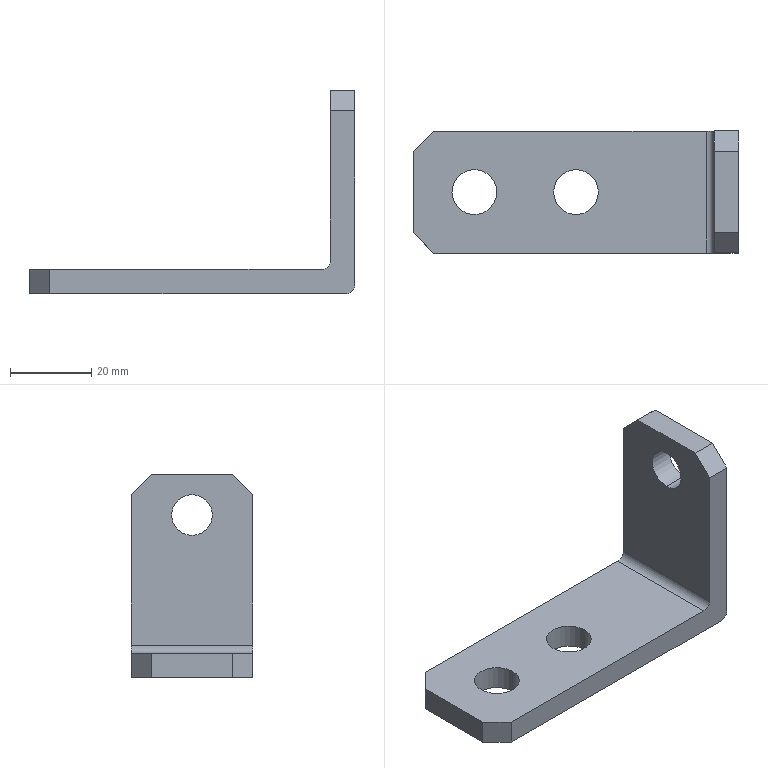Part | SolidWorks | features Chamfer 1, Extrusion 1, Fillet 1, ICE 1 | 1 solid | 20 faces | box 80 x 30 x 50 mm | volume 20408 mm3 | plane 12 | cylinder 8 | commonest cylinder face diameters 11 x4 4 x2 10 x2
STEP:
#1=CARTESIAN_POINT('',(34.,0.,45.));
#2=VERTEX_POINT('',#1);
#3=CARTESIAN_POINT('',(34.,0.,35.));
#4=VERTEX_POINT('',#3);
#5=CARTESIAN_POINT('',(34.,0.,40.));
#6=DIRECTION('',(1.,0.,0.));
#7=DIRECTION('',(0.,0.,-1.));
#8=AXIS2_PLACEMENT_3D('',#5,#6,#7);
#9=CIRCLE('',#8,5.);
#10=EDGE_CURVE('',#2,#4,#9,.T.);
#11=ORIENTED_EDGE('',*,*,#10,.F.);
#12=CARTESIAN_POINT('',(40.,0.,45.));
#13=VERTEX_POINT('',#12);
#14=CARTESIAN_POINT('',(34.,0.,45.));
#15=DIRECTION('',(1.,0.,0.));
#16=VECTOR('',#15,1000.);
#17=LINE('',#14,#16);
#18=EDGE_CURVE('',#2,#13,#17,.T.);
#19=ORIENTED_EDGE('',*,*,#18,.T.);
#20=CARTESIAN_POINT('',(40.,0.,35.));
#21=VERTEX_POINT('',#20);
#22=CARTESIAN_POINT('',(40.,0.,40.));
#23=DIRECTION('',(1.,0.,0.));
#24=DIRECTION('',(0.,0.,-1.));
#25=AXIS2_PLACEMENT_3D('',#22,#23,#24);
#26=CIRCLE('',#25,5.);
#27=EDGE_CURVE('',#13,#21,#26,.T.);
#28=ORIENTED_EDGE('',*,*,#27,.T.);
#29=CARTESIAN_POINT('',(34.,0.,35.));
#30=DIRECTION('',(1.,0.,0.));
#31=VECTOR('',#30,1000.);
#32=LINE('',#29,#31);
#33=EDGE_CURVE('',#4,#21,#32,.T.);
#34=ORIENTED_EDGE('',*,*,#33,.F.);
#35=EDGE_LOOP('',(#11,#19,#28,#34));
#36=FACE_OUTER_BOUND('',#35,.T.);
#37=CARTESIAN_POINT('',(34.,0.,40.));
#38=DIRECTION('',(1.,0.,0.));
#39=DIRECTION('',(0.,0.,-1.));
#40=AXIS2_PLACEMENT_3D('',#37,#38,#39);
#41=CYLINDRICAL_SURFACE('',#40,5.);
#42=ADVANCED_FACE('',(#36),#41,.F.);
#43=CARTESIAN_POINT('',(-30.5,0.,6.));
#44=VERTEX_POINT('',#43);
#45=CARTESIAN_POINT('',(-19.5,0.,6.));
#46=VERTEX_POINT('',#45);
#47=CARTESIAN_POINT('',(-25.,0.,6.));
#48=DIRECTION('',(0.,0.,1.));
#49=DIRECTION('',(1.,0.,0.));
#50=AXIS2_PLACEMENT_3D('',#47,#48,#49);
#51=CIRCLE('',#50,5.5);
#52=EDGE_CURVE('',#44,#46,#51,.T.);
#53=ORIENTED_EDGE('',*,*,#52,.T.);
#54=CARTESIAN_POINT('',(-19.5,0.,0.));
#55=VERTEX_POINT('',#54);
#56=CARTESIAN_POINT('',(-19.5,0.,6.));
#57=DIRECTION('',(0.,0.,-1.));
#58=VECTOR('',#57,1000.);
#59=LINE('',#56,#58);
#60=EDGE_CURVE('',#46,#55,#59,.T.);
#61=ORIENTED_EDGE('',*,*,#60,.T.);
#62=CARTESIAN_POINT('',(-30.5,0.,0.));
#63=VERTEX_POINT('',#62);
#64=CARTESIAN_POINT('',(-25.,0.,0.));
#65=DIRECTION('',(0.,0.,1.));
#66=DIRECTION('',(1.,0.,0.));
#67=AXIS2_PLACEMENT_3D('',#64,#65,#66);
#68=CIRCLE('',#67,5.5);
#69=EDGE_CURVE('',#63,#55,#68,.T.);
#70=ORIENTED_EDGE('',*,*,#69,.F.);
#71=CARTESIAN_POINT('',(-30.5,0.,6.));
#72=DIRECTION('',(0.,0.,-1.));
#73=VECTOR('',#72,1000.);
#74=LINE('',#71,#73);
#75=EDGE_CURVE('',#44,#63,#74,.T.);
#76=ORIENTED_EDGE('',*,*,#75,.F.);
#77=EDGE_LOOP('',(#53,#61,#70,#76));
#78=FACE_OUTER_BOUND('',#77,.T.);
#79=CARTESIAN_POINT('',(-25.,0.,6.));
#80=DIRECTION('',(0.,0.,-1.));
#81=DIRECTION('',(-1.,0.,0.));
#82=AXIS2_PLACEMENT_3D('',#79,#80,#81);
#83=CYLINDRICAL_SURFACE('',#82,5.5);
#84=ADVANCED_FACE('',(#78),#83,.F.);
#85=CARTESIAN_POINT('',(-5.5,0.,6.));
#86=VERTEX_POINT('',#85);
#87=CARTESIAN_POINT('',(5.5,0.,6.));
#88=VERTEX_POINT('',#87);
#89=CARTESIAN_POINT('',(0.,0.,6.));
#90=DIRECTION('',(0.,0.,1.));
#91=DIRECTION('',(1.,0.,0.));
#92=AXIS2_PLACEMENT_3D('',#89,#90,#91);
#93=CIRCLE('',#92,5.5);
#94=EDGE_CURVE('',#86,#88,#93,.T.);
#95=ORIENTED_EDGE('',*,*,#94,.T.);
#96=CARTESIAN_POINT('',(5.5,0.,0.));
#97=VERTEX_POINT('',#96);
#98=CARTESIAN_POINT('',(5.5,0.,6.));
#99=DIRECTION('',(0.,0.,-1.));
#100=VECTOR('',#99,1000.);
#101=LINE('',#98,#100);
#102=EDGE_CURVE('',#88,#97,#101,.T.);
#103=ORIENTED_EDGE('',*,*,#102,.T.);
#104=CARTESIAN_POINT('',(-5.5,0.,0.));
#105=VERTEX_POINT('',#104);
#106=CARTESIAN_POINT('',(0.,0.,0.));
#107=DIRECTION('',(0.,0.,1.));
#108=DIRECTION('',(1.,0.,0.));
#109=AXIS2_PLACEMENT_3D('',#106,#107,#108);
#110=CIRCLE('',#109,5.5);
#111=EDGE_CURVE('',#105,#97,#110,.T.);
#112=ORIENTED_EDGE('',*,*,#111,.F.);
#113=CARTESIAN_POINT('',(-5.5,0.,6.));
#114=DIRECTION('',(0.,0.,-1.));
#115=VECTOR('',#114,1000.);
#116=LINE('',#113,#115);
#117=EDGE_CURVE('',#86,#105,#116,.T.);
#118=ORIENTED_EDGE('',*,*,#117,.F.);
#119=EDGE_LOOP('',(#95,#103,#112,#118));
#120=FACE_OUTER_BOUND('',#119,.T.);
#121=CARTESIAN_POINT('',(0.,0.,6.));
#122=DIRECTION('',(0.,0.,-1.));
#123=DIRECTION('',(-1.,0.,0.));
#124=AXIS2_PLACEMENT_3D('',#121,#122,#123);
#125=CYLINDRICAL_SURFACE('',#124,5.5);
#126=ADVANCED_FACE('',(#120),#125,.F.);
#127=ORIENTED_EDGE('',*,*,#94,.F.);
#128=CARTESIAN_POINT('',(0.,0.,6.));
#129=DIRECTION('',(0.,0.,1.));
#130=DIRECTION('',(1.,0.,0.));
#131=AXIS2_PLACEMENT_3D('',#128,#129,#130);
#132=CIRCLE('',#131,5.5);
#133=EDGE_CURVE('',#88,#86,#132,.T.);
#134=ORIENTED_EDGE('',*,*,#133,.F.);
#135=EDGE_LOOP('',(#127,#134));
#136=FACE_BOUND('',#135,.T.);
#137=ORIENTED_EDGE('',*,*,#52,.F.);
#138=CARTESIAN_POINT('',(-25.,0.,6.));
#139=DIRECTION('',(0.,0.,1.));
#140=DIRECTION('',(1.,0.,0.));
#141=AXIS2_PLACEMENT_3D('',#138,#139,#140);
#142=CIRCLE('',#141,5.5);
#143=EDGE_CURVE('',#46,#44,#142,.T.);
#144=ORIENTED_EDGE('',*,*,#143,.F.);
#145=EDGE_LOOP('',(#137,#144));
#146=FACE_BOUND('',#145,.T.);
#147=CARTESIAN_POINT('',(-40.,10.,6.));
#148=VERTEX_POINT('',#147);
#149=CARTESIAN_POINT('',(-40.,-10.,6.));
#150=VERTEX_POINT('',#149);
#151=CARTESIAN_POINT('',(-40.,15.,6.));
#152=DIRECTION('',(0.,-1.,0.));
#153=VECTOR('',#152,1000.);
#154=LINE('',#151,#153);
#155=EDGE_CURVE('',#148,#150,#154,.T.);
#156=ORIENTED_EDGE('',*,*,#155,.T.);
#157=CARTESIAN_POINT('',(-35.,-15.,6.));
#158=VERTEX_POINT('',#157);
#159=CARTESIAN_POINT('',(-25.,-25.,6.));
#160=DIRECTION('',(0.7071,-0.7071,0.));
#161=VECTOR('',#160,1000.);
#162=LINE('',#159,#161);
#163=EDGE_CURVE('',#150,#158,#162,.T.);
#164=ORIENTED_EDGE('',*,*,#163,.T.);
#165=CARTESIAN_POINT('',(32.,-15.,6.));
#166=VERTEX_POINT('',#165);
#167=CARTESIAN_POINT('',(-40.,-15.,6.));
#168=DIRECTION('',(1.,0.,0.));
#169=VECTOR('',#168,1000.);
#170=LINE('',#167,#169);
#171=EDGE_CURVE('',#158,#166,#170,.T.);
#172=ORIENTED_EDGE('',*,*,#171,.T.);
#173=CARTESIAN_POINT('',(32.,15.,6.));
#174=VERTEX_POINT('',#173);
#175=CARTESIAN_POINT('',(32.,0.,6.));
#176=DIRECTION('',(0.,1.,0.));
#177=VECTOR('',#176,1000.);
#178=LINE('',#175,#177);
#179=EDGE_CURVE('',#166,#174,#178,.T.);
#180=ORIENTED_EDGE('',*,*,#179,.T.);
#181=CARTESIAN_POINT('',(-35.,15.,6.));
#182=VERTEX_POINT('',#181);
#183=CARTESIAN_POINT('',(-40.,15.,6.));
#184=DIRECTION('',(-1.,0.,0.));
#185=VECTOR('',#184,1000.);
#186=LINE('',#183,#185);
#187=EDGE_CURVE('',#174,#182,#186,.T.);
#188=ORIENTED_EDGE('',*,*,#187,.T.);
#189=CARTESIAN_POINT('',(-25.,25.,6.));
#190=DIRECTION('',(-0.7071,-0.7071,0.));
#191=VECTOR('',#190,1000.);
#192=LINE('',#189,#191);
#193=EDGE_CURVE('',#182,#148,#192,.T.);
#194=ORIENTED_EDGE('',*,*,#193,.T.);
#195=EDGE_LOOP('',(#156,#164,#172,#180,#188,#194));
#196=FACE_OUTER_BOUND('',#195,.T.);
#197=CARTESIAN_POINT('',(0.,0.,6.));
#198=DIRECTION('',(0.,0.,1.));
#199=DIRECTION('',(1.,0.,0.));
#200=AXIS2_PLACEMENT_3D('',#197,#198,#199);
#201=PLANE('',#200);
#202=ADVANCED_FACE('',(#136,#146,#196),#201,.T.);
#203=CARTESIAN_POINT('',(-35.,-15.,0.));
#204=VERTEX_POINT('',#203);
#205=CARTESIAN_POINT('',(38.,-15.,0.));
#206=VERTEX_POINT('',#205);
#207=CARTESIAN_POINT('',(-40.,-15.,0.));
#208=DIRECTION('',(1.,0.,0.));
#209=VECTOR('',#208,1000.);
#210=LINE('',#207,#209);
#211=EDGE_CURVE('',#204,#206,#210,.T.);
#212=ORIENTED_EDGE('',*,*,#211,.F.);
#213=CARTESIAN_POINT('',(-40.,-10.,0.));
#214=VERTEX_POINT('',#213);
#215=CARTESIAN_POINT('',(-35.,-15.,0.));
#216=DIRECTION('',(-0.7071,0.7071,0.));
#217=VECTOR('',#216,1000.);
#218=LINE('',#215,#217);
#219=EDGE_CURVE('',#204,#214,#218,.T.);
#220=ORIENTED_EDGE('',*,*,#219,.T.);
#221=CARTESIAN_POINT('',(-40.,10.,0.));
#222=VERTEX_POINT('',#221);
#223=CARTESIAN_POINT('',(-40.,15.,0.));
#224=DIRECTION('',(0.,-1.,0.));
#225=VECTOR('',#224,1000.);
#226=LINE('',#223,#225);
#227=EDGE_CURVE('',#222,#214,#226,.T.);
#228=ORIENTED_EDGE('',*,*,#227,.F.);
#229=CARTESIAN_POINT('',(-35.,15.,0.));
#230=VERTEX_POINT('',#229);
#231=CARTESIAN_POINT('',(-40.,10.,0.));
#232=DIRECTION('',(0.7071,0.7071,0.));
#233=VECTOR('',#232,1000.);
#234=LINE('',#231,#233);
#235=EDGE_CURVE('',#222,#230,#234,.T.);
#236=ORIENTED_EDGE('',*,*,#235,.T.);
#237=CARTESIAN_POINT('',(38.,15.,0.));
#238=VERTEX_POINT('',#237);
#239=CARTESIAN_POINT('',(-40.,15.,0.));
#240=DIRECTION('',(-1.,0.,0.));
#241=VECTOR('',#240,1000.);
#242=LINE('',#239,#241);
#243=EDGE_CURVE('',#238,#230,#242,.T.);
#244=ORIENTED_EDGE('',*,*,#243,.F.);
#245=CARTESIAN_POINT('',(38.,0.,0.));
#246=DIRECTION('',(0.,-1.,0.));
#247=VECTOR('',#246,1000.);
#248=LINE('',#245,#247);
#249=EDGE_CURVE('',#238,#206,#248,.T.);
#250=ORIENTED_EDGE('',*,*,#249,.T.);
#251=EDGE_LOOP('',(#212,#220,#228,#236,#244,#250));
#252=FACE_OUTER_BOUND('',#251,.T.);
#253=ORIENTED_EDGE('',*,*,#69,.T.);
#254=CARTESIAN_POINT('',(-25.,0.,0.));
#255=DIRECTION('',(0.,0.,1.));
#256=DIRECTION('',(1.,0.,0.));
#257=AXIS2_PLACEMENT_3D('',#254,#255,#256);
#258=CIRCLE('',#257,5.5);
#259=EDGE_CURVE('',#55,#63,#258,.T.);
#260=ORIENTED_EDGE('',*,*,#259,.T.);
#261=EDGE_LOOP('',(#253,#260));
#262=FACE_BOUND('',#261,.T.);
#263=ORIENTED_EDGE('',*,*,#111,.T.);
#264=CARTESIAN_POINT('',(0.,0.,0.));
#265=DIRECTION('',(0.,0.,1.));
#266=DIRECTION('',(1.,0.,0.));
#267=AXIS2_PLACEMENT_3D('',#264,#265,#266);
#268=CIRCLE('',#267,5.5);
#269=EDGE_CURVE('',#97,#105,#268,.T.);
#270=ORIENTED_EDGE('',*,*,#269,.T.);
#271=EDGE_LOOP('',(#263,#270));
#272=FACE_BOUND('',#271,.T.);
#273=CARTESIAN_POINT('',(0.,0.,0.));
#274=DIRECTION('',(0.,0.,1.));
#275=DIRECTION('',(1.,0.,0.));
#276=AXIS2_PLACEMENT_3D('',#273,#274,#275);
#277=PLANE('',#276);
#278=ADVANCED_FACE('',(#252,#262,#272),#277,.F.);
#279=CARTESIAN_POINT('',(40.,15.,45.));
#280=VERTEX_POINT('',#279);
#281=CARTESIAN_POINT('',(40.,15.,2.));
#282=VERTEX_POINT('',#281);
#283=CARTESIAN_POINT('',(40.,15.,6.));
#284=DIRECTION('',(0.,0.,-1.));
#285=VECTOR('',#284,1000.);
#286=LINE('',#283,#285);
#287=EDGE_CURVE('',#280,#282,#286,.T.);
#288=ORIENTED_EDGE('',*,*,#287,.F.);
#289=CARTESIAN_POINT('',(40.,10.,50.));
#290=VERTEX_POINT('',#289);
#291=CARTESIAN_POINT('',(40.,15.,45.));
#292=DIRECTION('',(0.,-0.7071,0.7071));
#293=VECTOR('',#292,1000.);
#294=LINE('',#291,#293);
#295=EDGE_CURVE('',#280,#290,#294,.T.);
#296=ORIENTED_EDGE('',*,*,#295,.T.);
#297=CARTESIAN_POINT('',(40.,-10.,50.));
#298=VERTEX_POINT('',#297);
#299=CARTESIAN_POINT('',(40.,15.,50.));
#300=DIRECTION('',(0.,-1.,0.));
#301=VECTOR('',#300,1000.);
#302=LINE('',#299,#301);
#303=EDGE_CURVE('',#290,#298,#302,.T.);
#304=ORIENTED_EDGE('',*,*,#303,.T.);
#305=CARTESIAN_POINT('',(40.,-15.,45.));
#306=VERTEX_POINT('',#305);
#307=CARTESIAN_POINT('',(40.,-10.,50.));
#308=DIRECTION('',(0.,-0.7071,-0.7071));
#309=VECTOR('',#308,1000.);
#310=LINE('',#307,#309);
#311=EDGE_CURVE('',#298,#306,#310,.T.);
#312=ORIENTED_EDGE('',*,*,#311,.T.);
#313=CARTESIAN_POINT('',(40.,-15.,2.));
#314=VERTEX_POINT('',#313);
#315=CARTESIAN_POINT('',(40.,-15.,6.));
#316=DIRECTION('',(0.,0.,-1.));
#317=VECTOR('',#316,1000.);
#318=LINE('',#315,#317);
#319=EDGE_CURVE('',#306,#314,#318,.T.);
#320=ORIENTED_EDGE('',*,*,#319,.T.);
#321=CARTESIAN_POINT('',(40.,15.,2.));
#322=DIRECTION('',(0.,1.,0.));
#323=VECTOR('',#322,1000.);
#324=LINE('',#321,#323);
#325=EDGE_CURVE('',#314,#282,#324,.T.);
#326=ORIENTED_EDGE('',*,*,#325,.T.);
#327=EDGE_LOOP('',(#288,#296,#304,#312,#320,#326));
#328=FACE_OUTER_BOUND('',#327,.T.);
#329=CARTESIAN_POINT('',(40.,0.,40.));
#330=DIRECTION('',(1.,0.,0.));
#331=DIRECTION('',(0.,0.,-1.));
#332=AXIS2_PLACEMENT_3D('',#329,#330,#331);
#333=CIRCLE('',#332,5.);
#334=EDGE_CURVE('',#21,#13,#333,.T.);
#335=ORIENTED_EDGE('',*,*,#334,.F.);
#336=ORIENTED_EDGE('',*,*,#27,.F.);
#337=EDGE_LOOP('',(#335,#336));
#338=FACE_BOUND('',#337,.T.);
#339=CARTESIAN_POINT('',(40.,15.,6.));
#340=DIRECTION('',(-1.,0.,0.));
#341=DIRECTION('',(0.,-1.,0.));
#342=AXIS2_PLACEMENT_3D('',#339,#340,#341);
#343=PLANE('',#342);
#344=ADVANCED_FACE('',(#328,#338),#343,.F.);
#345=ORIENTED_EDGE('',*,*,#243,.T.);
#346=CARTESIAN_POINT('',(-35.,15.,6.));
#347=DIRECTION('',(0.,0.,1.));
#348=VECTOR('',#347,1000.);
#349=LINE('',#346,#348);
#350=EDGE_CURVE('',#230,#182,#349,.T.);
#351=ORIENTED_EDGE('',*,*,#350,.T.);
#352=ORIENTED_EDGE('',*,*,#187,.F.);
#353=CARTESIAN_POINT('',(34.,15.,8.));
#354=VERTEX_POINT('',#353);
#355=CARTESIAN_POINT('',(32.,15.,8.));
#356=DIRECTION('',(0.,-1.,0.));
#357=DIRECTION('',(0.,0.,-1.));
#358=AXIS2_PLACEMENT_3D('',#355,#356,#357);
#359=CIRCLE('',#358,2.);
#360=EDGE_CURVE('',#174,#354,#359,.T.);
#361=ORIENTED_EDGE('',*,*,#360,.T.);
#362=CARTESIAN_POINT('',(34.,15.,45.));
#363=VERTEX_POINT('',#362);
#364=CARTESIAN_POINT('',(34.,15.,0.));
#365=DIRECTION('',(0.,0.,1.));
#366=VECTOR('',#365,1000.);
#367=LINE('',#364,#366);
#368=EDGE_CURVE('',#354,#363,#367,.T.);
#369=ORIENTED_EDGE('',*,*,#368,.T.);
#370=CARTESIAN_POINT('',(40.,15.,45.));
#371=DIRECTION('',(1.,0.,0.));
#372=VECTOR('',#371,1000.);
#373=LINE('',#370,#372);
#374=EDGE_CURVE('',#363,#280,#373,.T.);
#375=ORIENTED_EDGE('',*,*,#374,.T.);
#376=ORIENTED_EDGE('',*,*,#287,.T.);
#377=CARTESIAN_POINT('',(38.,15.,2.));
#378=DIRECTION('',(0.,1.,0.));
#379=DIRECTION('',(0.,0.,-1.));
#380=AXIS2_PLACEMENT_3D('',#377,#378,#379);
#381=CIRCLE('',#380,2.);
#382=EDGE_CURVE('',#282,#238,#381,.T.);
#383=ORIENTED_EDGE('',*,*,#382,.T.);
#384=EDGE_LOOP('',(#345,#351,#352,#361,#369,#375,#376,#383));
#385=FACE_OUTER_BOUND('',#384,.T.);
#386=CARTESIAN_POINT('',(-40.,15.,6.));
#387=DIRECTION('',(0.,-1.,0.));
#388=DIRECTION('',(0.,0.,-1.));
#389=AXIS2_PLACEMENT_3D('',#386,#387,#388);
#390=PLANE('',#389);
#391=ADVANCED_FACE('',(#385),#390,.F.);
#392=ORIENTED_EDGE('',*,*,#227,.T.);
#393=CARTESIAN_POINT('',(-40.,-10.,6.));
#394=DIRECTION('',(0.,0.,1.));
#395=VECTOR('',#394,1000.);
#396=LINE('',#393,#395);
#397=EDGE_CURVE('',#214,#150,#396,.T.);
#398=ORIENTED_EDGE('',*,*,#397,.T.);
#399=ORIENTED_EDGE('',*,*,#155,.F.);
#400=CARTESIAN_POINT('',(-40.,10.,6.));
#401=DIRECTION('',(0.,0.,-1.));
#402=VECTOR('',#401,1000.);
#403=LINE('',#400,#402);
#404=EDGE_CURVE('',#148,#222,#403,.T.);
#405=ORIENTED_EDGE('',*,*,#404,.T.);
#406=EDGE_LOOP('',(#392,#398,#399,#405));
#407=FACE_OUTER_BOUND('',#406,.T.);
#408=CARTESIAN_POINT('',(-40.,15.,6.));
#409=DIRECTION('',(1.,0.,0.));
#410=DIRECTION('',(0.,1.,0.));
#411=AXIS2_PLACEMENT_3D('',#408,#409,#410);
#412=PLANE('',#411);
#413=ADVANCED_FACE('',(#407),#412,.F.);
#414=ORIENTED_EDGE('',*,*,#171,.F.);
#415=CARTESIAN_POINT('',(-35.,-15.,6.));
#416=DIRECTION('',(0.,0.,-1.));
#417=VECTOR('',#416,1000.);
#418=LINE('',#415,#417);
#419=EDGE_CURVE('',#158,#204,#418,.T.);
#420=ORIENTED_EDGE('',*,*,#419,.T.);
#421=ORIENTED_EDGE('',*,*,#211,.T.);
#422=CARTESIAN_POINT('',(38.,-15.,2.));
#423=DIRECTION('',(0.,-1.,0.));
#424=DIRECTION('',(0.,0.,1.));
#425=AXIS2_PLACEMENT_3D('',#422,#423,#424);
#426=CIRCLE('',#425,2.);
#427=EDGE_CURVE('',#206,#314,#426,.T.);
#428=ORIENTED_EDGE('',*,*,#427,.T.);
#429=ORIENTED_EDGE('',*,*,#319,.F.);
#430=CARTESIAN_POINT('',(34.,-15.,45.));
#431=VERTEX_POINT('',#430);
#432=CARTESIAN_POINT('',(34.,-15.,45.));
#433=DIRECTION('',(-1.,0.,0.));
#434=VECTOR('',#433,1000.);
#435=LINE('',#432,#434);
#436=EDGE_CURVE('',#306,#431,#435,.T.);
#437=ORIENTED_EDGE('',*,*,#436,.T.);
#438=CARTESIAN_POINT('',(34.,-15.,8.));
#439=VERTEX_POINT('',#438);
#440=CARTESIAN_POINT('',(34.,-15.,0.));
#441=DIRECTION('',(0.,0.,-1.));
#442=VECTOR('',#441,1000.);
#443=LINE('',#440,#442);
#444=EDGE_CURVE('',#431,#439,#443,.T.);
#445=ORIENTED_EDGE('',*,*,#444,.T.);
#446=CARTESIAN_POINT('',(32.,-15.,8.));
#447=DIRECTION('',(0.,1.,0.));
#448=DIRECTION('',(0.,0.,1.));
#449=AXIS2_PLACEMENT_3D('',#446,#447,#448);
#450=CIRCLE('',#449,2.);
#451=EDGE_CURVE('',#439,#166,#450,.T.);
#452=ORIENTED_EDGE('',*,*,#451,.T.);
#453=EDGE_LOOP('',(#414,#420,#421,#428,#429,#437,#445,#452));
#454=FACE_OUTER_BOUND('',#453,.T.);
#455=CARTESIAN_POINT('',(-40.,-15.,6.));
#456=DIRECTION('',(0.,1.,0.));
#457=DIRECTION('',(0.,0.,1.));
#458=AXIS2_PLACEMENT_3D('',#455,#456,#457);
#459=PLANE('',#458);
#460=ADVANCED_FACE('',(#454),#459,.F.);
#461=ORIENTED_EDGE('',*,*,#102,.F.);
#462=ORIENTED_EDGE('',*,*,#133,.T.);
#463=ORIENTED_EDGE('',*,*,#117,.T.);
#464=ORIENTED_EDGE('',*,*,#269,.F.);
#465=EDGE_LOOP('',(#461,#462,#463,#464));
#466=FACE_OUTER_BOUND('',#465,.T.);
#467=CARTESIAN_POINT('',(0.,0.,6.));
#468=DIRECTION('',(0.,0.,-1.));
#469=DIRECTION('',(-1.,0.,0.));
#470=AXIS2_PLACEMENT_3D('',#467,#468,#469);
#471=CYLINDRICAL_SURFACE('',#470,5.5);
#472=ADVANCED_FACE('',(#466),#471,.F.);
#473=ORIENTED_EDGE('',*,*,#60,.F.);
#474=ORIENTED_EDGE('',*,*,#143,.T.);
#475=ORIENTED_EDGE('',*,*,#75,.T.);
#476=ORIENTED_EDGE('',*,*,#259,.F.);
#477=EDGE_LOOP('',(#473,#474,#475,#476));
#478=FACE_OUTER_BOUND('',#477,.T.);
#479=CARTESIAN_POINT('',(-25.,0.,6.));
#480=DIRECTION('',(0.,0.,-1.));
#481=DIRECTION('',(-1.,0.,0.));
#482=AXIS2_PLACEMENT_3D('',#479,#480,#481);
#483=CYLINDRICAL_SURFACE('',#482,5.5);
#484=ADVANCED_FACE('',(#478),#483,.F.);
#485=ORIENTED_EDGE('',*,*,#303,.F.);
#486=CARTESIAN_POINT('',(34.,10.,50.));
#487=VERTEX_POINT('',#486);
#488=CARTESIAN_POINT('',(34.,10.,50.));
#489=DIRECTION('',(-1.,0.,0.));
#490=VECTOR('',#489,1000.);
#491=LINE('',#488,#490);
#492=EDGE_CURVE('',#290,#487,#491,.T.);
#493=ORIENTED_EDGE('',*,*,#492,.T.);
#494=CARTESIAN_POINT('',(34.,-10.,50.));
#495=VERTEX_POINT('',#494);
#496=CARTESIAN_POINT('',(34.,15.,50.));
#497=DIRECTION('',(0.,-1.,0.));
#498=VECTOR('',#497,1000.);
#499=LINE('',#496,#498);
#500=EDGE_CURVE('',#487,#495,#499,.T.);
#501=ORIENTED_EDGE('',*,*,#500,.T.);
#502=CARTESIAN_POINT('',(40.,-10.,50.));
#503=DIRECTION('',(1.,0.,0.));
#504=VECTOR('',#503,1000.);
#505=LINE('',#502,#504);
#506=EDGE_CURVE('',#495,#298,#505,.T.);
#507=ORIENTED_EDGE('',*,*,#506,.T.);
#508=EDGE_LOOP('',(#485,#493,#501,#507));
#509=FACE_OUTER_BOUND('',#508,.T.);
#510=CARTESIAN_POINT('',(34.,15.,50.));
#511=DIRECTION('',(0.,0.,1.));
#512=DIRECTION('',(0.,-1.,0.));
#513=AXIS2_PLACEMENT_3D('',#510,#511,#512);
#514=PLANE('',#513);
#515=ADVANCED_FACE('',(#509),#514,.T.);
#516=ORIENTED_EDGE('',*,*,#500,.F.);
#517=CARTESIAN_POINT('',(34.,15.,45.));
#518=DIRECTION('',(0.,0.7071,-0.7071));
#519=VECTOR('',#518,1000.);
#520=LINE('',#517,#519);
#521=EDGE_CURVE('',#487,#363,#520,.T.);
#522=ORIENTED_EDGE('',*,*,#521,.T.);
#523=ORIENTED_EDGE('',*,*,#368,.F.);
#524=CARTESIAN_POINT('',(34.,0.,8.));
#525=DIRECTION('',(0.,-1.,0.));
#526=VECTOR('',#525,1000.);
#527=LINE('',#524,#526);
#528=EDGE_CURVE('',#354,#439,#527,.T.);
#529=ORIENTED_EDGE('',*,*,#528,.T.);
#530=ORIENTED_EDGE('',*,*,#444,.F.);
#531=CARTESIAN_POINT('',(34.,-10.,50.));
#532=DIRECTION('',(0.,0.7071,0.7071));
#533=VECTOR('',#532,1000.);
#534=LINE('',#531,#533);
#535=EDGE_CURVE('',#431,#495,#534,.T.);
#536=ORIENTED_EDGE('',*,*,#535,.T.);
#537=EDGE_LOOP('',(#516,#522,#523,#529,#530,#536));
#538=FACE_OUTER_BOUND('',#537,.T.);
#539=CARTESIAN_POINT('',(34.,0.,40.));
#540=DIRECTION('',(1.,0.,0.));
#541=DIRECTION('',(0.,0.,-1.));
#542=AXIS2_PLACEMENT_3D('',#539,#540,#541);
#543=CIRCLE('',#542,5.);
#544=EDGE_CURVE('',#4,#2,#543,.T.);
#545=ORIENTED_EDGE('',*,*,#544,.T.);
#546=ORIENTED_EDGE('',*,*,#10,.T.);
#547=EDGE_LOOP('',(#545,#546));
#548=FACE_BOUND('',#547,.T.);
#549=CARTESIAN_POINT('',(34.,0.,0.));
#550=DIRECTION('',(1.,0.,0.));
#551=DIRECTION('',(0.,0.,-1.));
#552=AXIS2_PLACEMENT_3D('',#549,#550,#551);
#553=PLANE('',#552);
#554=ADVANCED_FACE('',(#538,#548),#553,.F.);
#555=ORIENTED_EDGE('',*,*,#18,.F.);
#556=ORIENTED_EDGE('',*,*,#544,.F.);
#557=ORIENTED_EDGE('',*,*,#33,.T.);
#558=ORIENTED_EDGE('',*,*,#334,.T.);
#559=EDGE_LOOP('',(#555,#556,#557,#558));
#560=FACE_OUTER_BOUND('',#559,.T.);
#561=CARTESIAN_POINT('',(34.,0.,40.));
#562=DIRECTION('',(1.,0.,0.));
#563=DIRECTION('',(0.,0.,-1.));
#564=AXIS2_PLACEMENT_3D('',#561,#562,#563);
#565=CYLINDRICAL_SURFACE('',#564,5.);
#566=ADVANCED_FACE('',(#560),#565,.F.);
#567=ORIENTED_EDGE('',*,*,#427,.F.);
#568=ORIENTED_EDGE('',*,*,#249,.F.);
#569=ORIENTED_EDGE('',*,*,#382,.F.);
#570=ORIENTED_EDGE('',*,*,#325,.F.);
#571=EDGE_LOOP('',(#567,#568,#569,#570));
#572=FACE_OUTER_BOUND('',#571,.T.);
#573=CARTESIAN_POINT('',(38.,15.,2.));
#574=DIRECTION('',(0.,1.,0.));
#575=DIRECTION('',(-1.,0.,0.));
#576=AXIS2_PLACEMENT_3D('',#573,#574,#575);
#577=CYLINDRICAL_SURFACE('',#576,2.);
#578=ADVANCED_FACE('',(#572),#577,.T.);
#579=ORIENTED_EDGE('',*,*,#451,.F.);
#580=ORIENTED_EDGE('',*,*,#528,.F.);
#581=ORIENTED_EDGE('',*,*,#360,.F.);
#582=ORIENTED_EDGE('',*,*,#179,.F.);
#583=EDGE_LOOP('',(#579,#580,#581,#582));
#584=FACE_OUTER_BOUND('',#583,.T.);
#585=CARTESIAN_POINT('',(32.,0.,8.));
#586=DIRECTION('',(0.,1.,0.));
#587=DIRECTION('',(0.,0.,1.));
#588=AXIS2_PLACEMENT_3D('',#585,#586,#587);
#589=CYLINDRICAL_SURFACE('',#588,2.);
#590=ADVANCED_FACE('',(#584),#589,.F.);
#591=ORIENTED_EDGE('',*,*,#163,.F.);
#592=ORIENTED_EDGE('',*,*,#397,.F.);
#593=ORIENTED_EDGE('',*,*,#219,.F.);
#594=ORIENTED_EDGE('',*,*,#419,.F.);
#595=EDGE_LOOP('',(#591,#592,#593,#594));
#596=FACE_OUTER_BOUND('',#595,.T.);
#597=CARTESIAN_POINT('',(-35.,-15.,6.));
#598=DIRECTION('',(0.7071,0.7071,0.));
#599=DIRECTION('',(0.,0.,-1.));
#600=AXIS2_PLACEMENT_3D('',#597,#598,#599);
#601=PLANE('',#600);
#602=ADVANCED_FACE('',(#596),#601,.F.);
#603=ORIENTED_EDGE('',*,*,#193,.F.);
#604=ORIENTED_EDGE('',*,*,#350,.F.);
#605=ORIENTED_EDGE('',*,*,#235,.F.);
#606=ORIENTED_EDGE('',*,*,#404,.F.);
#607=EDGE_LOOP('',(#603,#604,#605,#606));
#608=FACE_OUTER_BOUND('',#607,.T.);
#609=CARTESIAN_POINT('',(-40.,10.,6.));
#610=DIRECTION('',(0.7071,-0.7071,0.));
#611=DIRECTION('',(0.,0.,-1.));
#612=AXIS2_PLACEMENT_3D('',#609,#610,#611);
#613=PLANE('',#612);
#614=ADVANCED_FACE('',(#608),#613,.F.);
#615=ORIENTED_EDGE('',*,*,#521,.F.);
#616=ORIENTED_EDGE('',*,*,#492,.F.);
#617=ORIENTED_EDGE('',*,*,#295,.F.);
#618=ORIENTED_EDGE('',*,*,#374,.F.);
#619=EDGE_LOOP('',(#615,#616,#617,#618));
#620=FACE_OUTER_BOUND('',#619,.T.);
#621=CARTESIAN_POINT('',(-40.,15.,45.));
#622=DIRECTION('',(0.,0.7071,0.7071));
#623=DIRECTION('',(-1.,0.,0.));
#624=AXIS2_PLACEMENT_3D('',#621,#622,#623);
#625=PLANE('',#624);
#626=ADVANCED_FACE('',(#620),#625,.T.);
#627=ORIENTED_EDGE('',*,*,#535,.F.);
#628=ORIENTED_EDGE('',*,*,#436,.F.);
#629=ORIENTED_EDGE('',*,*,#311,.F.);
#630=ORIENTED_EDGE('',*,*,#506,.F.);
#631=EDGE_LOOP('',(#627,#628,#629,#630));
#632=FACE_OUTER_BOUND('',#631,.T.);
#633=CARTESIAN_POINT('',(34.,-10.,50.));
#634=DIRECTION('',(0.,-0.7071,0.7071));
#635=DIRECTION('',(-1.,0.,0.));
#636=AXIS2_PLACEMENT_3D('',#633,#634,#635);
#637=PLANE('',#636);
#638=ADVANCED_FACE('',(#632),#637,.T.);
#639=CLOSED_SHELL('',(#42,#84,#126,#202,#278,#344,#391,#413,#460,#472,#484,#515,#554,#566,#578,#590,#602,#614,#626,#638));
#640=MANIFOLD_SOLID_BREP('',#639);
#641=CARTESIAN_POINT('',(0.,0.,0.));
#642=DIRECTION('',(0.,0.,1.));
#643=DIRECTION('',(1.,0.,0.));
#644=AXIS2_PLACEMENT_3D('',#641,#642,#643);
#645=(LENGTH_UNIT()NAMED_UNIT(*)SI_UNIT(.MILLI.,.METRE.));
#646=UNCERTAINTY_MEASURE_WITH_UNIT(LENGTH_MEASURE(0.00001),#645,'','');
#647=(NAMED_UNIT(*)PLANE_ANGLE_UNIT()SI_UNIT($,.RADIAN.));
#648=(NAMED_UNIT(*)SI_UNIT($,.STERADIAN.)SOLID_ANGLE_UNIT());
#649=(GEOMETRIC_REPRESENTATION_CONTEXT(3)GLOBAL_UNCERTAINTY_ASSIGNED_CONTEXT((#646))GLOBAL_UNIT_ASSIGNED_CONTEXT((#645,#647,#648))REPRESENTATION_CONTEXT('',''));
#650=ADVANCED_BREP_SHAPE_REPRESENTATION('',(#640,#644),#649);